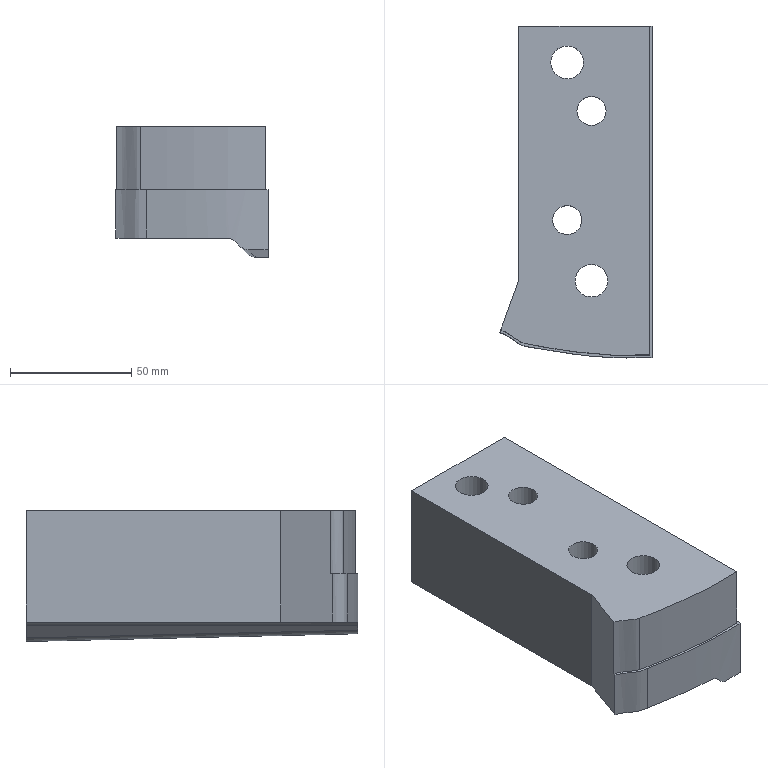Part | NX | features solid 2 | 1 solid | 30 faces | box 62.75 x 136.771 x 54 mm | volume 322596 mm3 | plane 16 | cylinder 10 | spline 4 | commonest cylinder face diameters 10 x2 12 x2 13 x2 13.5 x2 19.5 x2
STEP:
#1=CARTESIAN_POINT('',(-125.,123.027,40.));
#2=VERTEX_POINT('',#1);
#3=CARTESIAN_POINT('',(-125.,123.027,-6.));
#4=VERTEX_POINT('',#3);
#5=CARTESIAN_POINT('',(-125.,123.027,23.));
#6=DIRECTION('',(0.,0.,-1.));
#7=VECTOR('',#6,1000.);
#8=LINE('',#5,#7);
#9=EDGE_CURVE('',#2,#4,#8,.T.);
#10=ORIENTED_EDGE('',*,*,#9,.F.);
#11=CARTESIAN_POINT('',(-125.,228.,40.));
#12=VERTEX_POINT('',#11);
#13=CARTESIAN_POINT('',(-125.,35.09,40.));
#14=DIRECTION('',(0.,1.,0.));
#15=VECTOR('',#14,1000.);
#16=LINE('',#13,#15);
#17=EDGE_CURVE('',#2,#12,#16,.T.);
#18=ORIENTED_EDGE('',*,*,#17,.T.);
#19=CARTESIAN_POINT('',(-125.,228.,-6.));
#20=VERTEX_POINT('',#19);
#21=CARTESIAN_POINT('',(-125.,228.,-206.));
#22=DIRECTION('',(0.,0.,1.));
#23=VECTOR('',#22,1000.);
#24=LINE('',#21,#23);
#25=EDGE_CURVE('',#20,#12,#24,.T.);
#26=ORIENTED_EDGE('',*,*,#25,.F.);
#27=CARTESIAN_POINT('',(-125.,-222.,-6.));
#28=DIRECTION('',(0.,-1.,0.));
#29=VECTOR('',#28,1000.);
#30=LINE('',#27,#29);
#31=EDGE_CURVE('',#20,#4,#30,.T.);
#32=ORIENTED_EDGE('',*,*,#31,.T.);
#33=EDGE_LOOP('',(#10,#18,#26,#32));
#34=FACE_BOUND('',#33,.T.);
#35=CARTESIAN_POINT('',(-125.,163.62,23.));
#36=DIRECTION('',(1.,0.,0.));
#37=DIRECTION('',(0.,0.,-1.));
#38=AXIS2_PLACEMENT_3D('',#35,#36,#37);
#39=PLANE('',#38);
#40=ADVANCED_FACE('',(#34),#39,.F.);
#41=CARTESIAN_POINT('',(-71.,92.393,40.));
#42=VERTEX_POINT('',#41);
#43=CARTESIAN_POINT('',(-122.771,97.196,40.));
#44=VERTEX_POINT('',#43);
#45=CARTESIAN_POINT('',(-71.,92.393,40.));
#46=CARTESIAN_POINT('',(-75.359,92.271,40.));
#47=CARTESIAN_POINT('',(-84.076,92.056,40.));
#48=CARTESIAN_POINT('',(-97.043,93.007,40.));
#49=CARTESIAN_POINT('',(-109.924,94.861,40.));
#50=CARTESIAN_POINT('',(-118.523,96.209,40.));
#51=CARTESIAN_POINT('',(-122.771,97.196,40.));
#52=B_SPLINE_CURVE_WITH_KNOTS('',3,(#45,#46,#47,#48,#49,#50,#51),.UNSPECIFIED.,.F.,.F.,(4,1,1,1,4),(0.,0.013,0.026,0.039,0.052),.UNSPECIFIED.);
#53=EDGE_CURVE('',#42,#44,#52,.T.);
#54=ORIENTED_EDGE('',*,*,#53,.F.);
#55=CARTESIAN_POINT('',(-71.,228.,40.));
#56=VERTEX_POINT('',#55);
#57=CARTESIAN_POINT('',(-71.,35.09,40.));
#58=DIRECTION('',(0.,1.,0.));
#59=VECTOR('',#58,1000.);
#60=LINE('',#57,#59);
#61=EDGE_CURVE('',#42,#56,#60,.T.);
#62=ORIENTED_EDGE('',*,*,#61,.T.);
#63=CARTESIAN_POINT('',(-415.478,228.,40.));
#64=DIRECTION('',(1.,0.,0.));
#65=VECTOR('',#64,1000.);
#66=LINE('',#63,#65);
#67=EDGE_CURVE('',#12,#56,#66,.T.);
#68=ORIENTED_EDGE('',*,*,#67,.F.);
#69=ORIENTED_EDGE('',*,*,#17,.F.);
#70=CARTESIAN_POINT('',(-132.408,102.674,40.));
#71=VERTEX_POINT('',#70);
#72=CARTESIAN_POINT('',(-187.242,-47.981,40.));
#73=DIRECTION('',(0.342,0.9397,0.));
#74=VECTOR('',#73,1000.);
#75=LINE('',#72,#74);
#76=EDGE_CURVE('',#71,#2,#75,.T.);
#77=ORIENTED_EDGE('',*,*,#76,.F.);
#78=CARTESIAN_POINT('',(-122.771,97.196,40.));
#79=CARTESIAN_POINT('',(-124.596,97.621,40.));
#80=CARTESIAN_POINT('',(-126.742,99.529,40.));
#81=CARTESIAN_POINT('',(-129.792,101.652,40.));
#82=CARTESIAN_POINT('',(-131.523,102.356,40.));
#83=CARTESIAN_POINT('',(-132.408,102.674,40.));
#84=B_SPLINE_CURVE_WITH_KNOTS('',3,(#78,#79,#80,#81,#82,#83),.UNSPECIFIED.,.F.,.F.,(4,1,1,4),(0.,0.00551,0.008265,0.01102),.UNSPECIFIED.);
#85=EDGE_CURVE('',#44,#71,#84,.T.);
#86=ORIENTED_EDGE('',*,*,#85,.F.);
#87=EDGE_LOOP('',(#54,#62,#68,#69,#77,#86));
#88=FACE_BOUND('',#87,.T.);
#89=CARTESIAN_POINT('',(-89.,193.,40.));
#90=VERTEX_POINT('',#89);
#91=CARTESIAN_POINT('',(-95.,193.,40.));
#92=DIRECTION('',(0.,0.,1.));
#93=DIRECTION('',(1.,0.,0.));
#94=AXIS2_PLACEMENT_3D('',#91,#92,#93);
#95=CIRCLE('',#94,6.);
#96=EDGE_CURVE('',#90,#90,#95,.T.);
#97=ORIENTED_EDGE('',*,*,#96,.F.);
#98=EDGE_LOOP('',(#97));
#99=FACE_BOUND('',#98,.T.);
#100=CARTESIAN_POINT('',(-99.,148.,40.));
#101=VERTEX_POINT('',#100);
#102=CARTESIAN_POINT('',(-105.,148.,40.));
#103=DIRECTION('',(0.,0.,1.));
#104=DIRECTION('',(1.,0.,0.));
#105=AXIS2_PLACEMENT_3D('',#102,#103,#104);
#106=CIRCLE('',#105,6.);
#107=EDGE_CURVE('',#101,#101,#106,.T.);
#108=ORIENTED_EDGE('',*,*,#107,.F.);
#109=EDGE_LOOP('',(#108));
#110=FACE_BOUND('',#109,.T.);
#111=CARTESIAN_POINT('',(-98.25,213.,40.));
#112=VERTEX_POINT('',#111);
#113=CARTESIAN_POINT('',(-105.,213.,40.));
#114=DIRECTION('',(0.,0.,1.));
#115=DIRECTION('',(1.,0.,0.));
#116=AXIS2_PLACEMENT_3D('',#113,#114,#115);
#117=CIRCLE('',#116,6.75);
#118=EDGE_CURVE('',#112,#112,#117,.T.);
#119=ORIENTED_EDGE('',*,*,#118,.F.);
#120=EDGE_LOOP('',(#119));
#121=FACE_BOUND('',#120,.T.);
#122=CARTESIAN_POINT('',(-88.25,123.,40.));
#123=VERTEX_POINT('',#122);
#124=CARTESIAN_POINT('',(-95.,123.,40.));
#125=DIRECTION('',(0.,0.,1.));
#126=DIRECTION('',(1.,0.,0.));
#127=AXIS2_PLACEMENT_3D('',#124,#125,#126);
#128=CIRCLE('',#127,6.75);
#129=EDGE_CURVE('',#123,#123,#128,.T.);
#130=ORIENTED_EDGE('',*,*,#129,.F.);
#131=EDGE_LOOP('',(#130));
#132=FACE_BOUND('',#131,.T.);
#133=CARTESIAN_POINT('',(-415.478,35.09,40.));
#134=DIRECTION('',(0.,0.,1.));
#135=DIRECTION('',(1.,0.,0.));
#136=AXIS2_PLACEMENT_3D('',#133,#134,#135);
#137=PLANE('',#136);
#138=ADVANCED_FACE('',(#88,#99,#110,#121,#132),#137,.T.);
#139=CARTESIAN_POINT('',(-83.536,91.257,-7.464));
#140=VERTEX_POINT('',#139);
#141=CARTESIAN_POINT('',(-81.651,91.233,-9.349));
#142=VERTEX_POINT('',#141);
#143=CARTESIAN_POINT('',(-83.536,91.257,-7.464));
#144=CARTESIAN_POINT('',(-82.907,91.245,-8.093));
#145=CARTESIAN_POINT('',(-82.279,91.237,-8.721));
#146=CARTESIAN_POINT('',(-81.651,91.233,-9.349));
#147=B_SPLINE_CURVE_WITH_KNOTS('',3,(#143,#144,#145,#146),.UNSPECIFIED.,.F.,.F.,(4,4),(0.002071,0.004736),.UNSPECIFIED.);
#148=EDGE_CURVE('',#140,#142,#147,.T.);
#149=ORIENTED_EDGE('',*,*,#148,.T.);
#150=CARTESIAN_POINT('',(-78.112,91.242,-10.815));
#151=VERTEX_POINT('',#150);
#152=CARTESIAN_POINT('',(-81.651,91.233,-9.349));
#153=CARTESIAN_POINT('',(-80.717,91.226,-10.283));
#154=CARTESIAN_POINT('',(-79.433,91.228,-10.815));
#155=CARTESIAN_POINT('',(-78.112,91.242,-10.815));
#156=B_SPLINE_CURVE_WITH_KNOTS('',3,(#152,#153,#154,#155),.UNSPECIFIED.,.F.,.F.,(4,4),(0.,0.003908),.UNSPECIFIED.);
#157=EDGE_CURVE('',#142,#151,#156,.T.);
#158=ORIENTED_EDGE('',*,*,#157,.T.);
#159=CARTESIAN_POINT('',(-70.,91.421,-10.818));
#160=VERTEX_POINT('',#159);
#161=CARTESIAN_POINT('',(-78.112,91.242,-10.815));
#162=CARTESIAN_POINT('',(-75.407,91.271,-10.815));
#163=CARTESIAN_POINT('',(-72.704,91.343,-10.816));
#164=CARTESIAN_POINT('',(-70.,91.421,-10.818));
#165=B_SPLINE_CURVE_WITH_KNOTS('',3,(#161,#162,#163,#164),.UNSPECIFIED.,.F.,.F.,(4,4),(0.002073,0.01019),.UNSPECIFIED.);
#166=EDGE_CURVE('',#151,#160,#165,.T.);
#167=ORIENTED_EDGE('',*,*,#166,.T.);
#168=CARTESIAN_POINT('',(-70.,91.421,14.));
#169=VERTEX_POINT('',#168);
#170=CARTESIAN_POINT('',(-70.,91.421,1.5));
#171=DIRECTION('',(0.,0.,-1.));
#172=VECTOR('',#171,1000.);
#173=LINE('',#170,#172);
#174=EDGE_CURVE('',#169,#160,#173,.T.);
#175=ORIENTED_EDGE('',*,*,#174,.F.);
#176=CARTESIAN_POINT('',(-71.,91.392,14.));
#177=VERTEX_POINT('',#176);
#178=CARTESIAN_POINT('',(-71.,91.392,14.));
#179=CARTESIAN_POINT('',(-70.667,91.402,14.));
#180=CARTESIAN_POINT('',(-70.333,91.411,14.));
#181=CARTESIAN_POINT('',(-70.,91.421,14.));
#182=B_SPLINE_CURVE_WITH_KNOTS('',3,(#178,#179,#180,#181),.UNSPECIFIED.,.F.,.F.,(4,4),(0.04918,0.05017),.UNSPECIFIED.);
#183=EDGE_CURVE('',#177,#169,#182,.T.);
#184=ORIENTED_EDGE('',*,*,#183,.F.);
#185=CARTESIAN_POINT('',(-120.,95.579,14.));
#186=VERTEX_POINT('',#185);
#187=CARTESIAN_POINT('',(-190.231,-121.49,14.));
#188=CARTESIAN_POINT('',(-188.654,-121.152,14.));
#189=CARTESIAN_POINT('',(-185.47,-120.627,14.));
#190=CARTESIAN_POINT('',(-180.656,-120.141,14.));
#191=CARTESIAN_POINT('',(-175.882,-119.326,14.));
#192=CARTESIAN_POINT('',(-169.679,-117.528,14.));
#193=CARTESIAN_POINT('',(-162.185,-114.539,14.));
#194=CARTESIAN_POINT('',(-153.086,-111.254,14.));
#195=CARTESIAN_POINT('',(-144.031,-107.845,14.));
#196=CARTESIAN_POINT('',(-136.465,-105.061,14.));
#197=CARTESIAN_POINT('',(-130.418,-102.814,14.));
#198=CARTESIAN_POINT('',(-125.812,-101.329,14.));
#199=CARTESIAN_POINT('',(-121.306,-99.566,14.));
#200=CARTESIAN_POINT('',(-116.876,-97.626,14.));
#201=CARTESIAN_POINT('',(-112.335,-95.923,14.));
#202=CARTESIAN_POINT('',(-107.564,-95.05,14.));
#203=CARTESIAN_POINT('',(-102.756,-94.525,14.));
#204=CARTESIAN_POINT('',(-96.349,-93.771,14.));
#205=CARTESIAN_POINT('',(-89.902,-93.468,14.));
#206=CARTESIAN_POINT('',(-83.452,-93.448,14.));
#207=CARTESIAN_POINT('',(-77.002,-93.469,14.));
#208=CARTESIAN_POINT('',(-68.939,-93.411,14.));
#209=CARTESIAN_POINT('',(-56.04,-93.3,14.));
#210=CARTESIAN_POINT('',(-33.465,-93.184,14.));
#211=CARTESIAN_POINT('',(-7.666,-93.074,14.));
#212=CARTESIAN_POINT('',(14.907,-92.653,14.));
#213=CARTESIAN_POINT('',(27.794,-92.068,14.));
#214=CARTESIAN_POINT('',(40.668,-91.245,14.));
#215=CARTESIAN_POINT('',(51.917,-90.291,14.));
#216=CARTESIAN_POINT('',(61.528,-89.174,14.));
#217=CARTESIAN_POINT('',(67.939,-88.466,14.));
#218=CARTESIAN_POINT('',(79.125,-86.95,14.));
#219=CARTESIAN_POINT('',(95.161,-85.253,14.));
#220=CARTESIAN_POINT('',(114.404,-83.21,14.));
#221=CARTESIAN_POINT('',(133.568,-80.524,14.));
#222=CARTESIAN_POINT('',(152.734,-77.861,14.));
#223=CARTESIAN_POINT('',(171.916,-75.326,14.));
#224=CARTESIAN_POINT('',(191.055,-72.413,14.));
#225=CARTESIAN_POINT('',(207.17,-71.468,14.));
#226=CARTESIAN_POINT('',(219.951,-69.697,14.));
#227=CARTESIAN_POINT('',(232.724,-67.899,14.));
#228=CARTESIAN_POINT('',(248.708,-65.766,14.));
#229=CARTESIAN_POINT('',(267.87,-63.074,14.));
#230=CARTESIAN_POINT('',(287.038,-60.44,14.));
#231=CARTESIAN_POINT('',(301.448,-58.682,14.));
#232=CARTESIAN_POINT('',(310.976,-56.987,14.));
#233=CARTESIAN_POINT('',(314.916,-56.135,14.));
#234=CARTESIAN_POINT('',(318.052,-55.382,14.));
#235=CARTESIAN_POINT('',(320.39,-54.76,14.));
#236=CARTESIAN_POINT('',(322.686,-53.981,14.));
#237=CARTESIAN_POINT('',(325.595,-52.578,14.));
#238=CARTESIAN_POINT('',(328.769,-50.098,14.));
#239=CARTESIAN_POINT('',(332.247,-46.69,14.));
#240=CARTESIAN_POINT('',(335.795,-43.406,14.));
#241=CARTESIAN_POINT('',(343.661,-37.758,14.));
#242=CARTESIAN_POINT('',(355.164,-28.914,14.));
#243=CARTESIAN_POINT('',(370.422,-17.018,14.));
#244=CARTESIAN_POINT('',(383.264,-7.249,14.));
#245=CARTESIAN_POINT('',(392.416,-0.6713,14.));
#246=CARTESIAN_POINT('',(396.953,2.733,14.));
#247=CARTESIAN_POINT('',(398.886,5.372,14.));
#248=CARTESIAN_POINT('',(399.725,7.654,14.));
#249=CARTESIAN_POINT('',(399.76,10.078,14.));
#250=CARTESIAN_POINT('',(399.483,13.317,14.));
#251=CARTESIAN_POINT('',(399.712,17.34,14.));
#252=CARTESIAN_POINT('',(399.612,22.179,14.));
#253=CARTESIAN_POINT('',(399.633,31.854,14.));
#254=CARTESIAN_POINT('',(399.593,46.366,14.));
#255=CARTESIAN_POINT('',(399.637,62.491,14.));
#256=CARTESIAN_POINT('',(399.588,73.779,14.));
#257=CARTESIAN_POINT('',(399.652,79.422,14.));
#258=CARTESIAN_POINT('',(399.59,82.647,14.));
#259=CARTESIAN_POINT('',(399.564,85.065,14.));
#260=CARTESIAN_POINT('',(399.725,87.486,14.));
#261=CARTESIAN_POINT('',(399.756,89.902,14.));
#262=CARTESIAN_POINT('',(399.247,92.301,14.));
#263=CARTESIAN_POINT('',(397.362,95.008,14.));
#264=CARTESIAN_POINT('',(393.635,96.774,14.));
#265=CARTESIAN_POINT('',(389.279,98.826,14.));
#266=CARTESIAN_POINT('',(384.732,100.498,14.));
#267=CARTESIAN_POINT('',(378.765,102.95,14.));
#268=CARTESIAN_POINT('',(362.589,110.229,14.));
#269=CARTESIAN_POINT('',(344.928,118.135,14.));
#270=CARTESIAN_POINT('',(327.281,126.072,14.));
#271=CARTESIAN_POINT('',(319.932,129.381,14.));
#272=CARTESIAN_POINT('',(314.075,132.102,14.));
#273=CARTESIAN_POINT('',(309.387,133.376,14.));
#274=CARTESIAN_POINT('',(304.547,133.785,14.));
#275=CARTESIAN_POINT('',(299.716,133.401,14.));
#276=CARTESIAN_POINT('',(294.929,132.704,14.));
#277=CARTESIAN_POINT('',(288.543,131.8,14.));
#278=CARTESIAN_POINT('',(277.364,130.241,14.));
#279=CARTESIAN_POINT('',(242.2,125.552,14.));
#280=CARTESIAN_POINT('',(184.637,118.048,14.));
#281=CARTESIAN_POINT('',(120.701,109.541,14.));
#282=CARTESIAN_POINT('',(69.531,102.902,14.));
#283=CARTESIAN_POINT('',(40.777,98.94,14.));
#284=CARTESIAN_POINT('',(21.566,96.615,14.));
#285=CARTESIAN_POINT('',(8.743,95.212,14.));
#286=CARTESIAN_POINT('',(-7.301,93.575,14.));
#287=CARTESIAN_POINT('',(-26.625,92.505,14.));
#288=CARTESIAN_POINT('',(-45.971,92.017,14.));
#289=CARTESIAN_POINT('',(-62.09,91.675,14.));
#290=CARTESIAN_POINT('',(-74.987,91.256,14.));
#291=CARTESIAN_POINT('',(-84.664,91.165,14.));
#292=CARTESIAN_POINT('',(-94.319,91.781,14.));
#293=CARTESIAN_POINT('',(-103.929,92.966,14.));
#294=CARTESIAN_POINT('',(-113.495,94.403,14.));
#295=CARTESIAN_POINT('',(-119.856,95.492,14.));
#296=CARTESIAN_POINT('',(-122.997,96.222,14.));
#297=B_SPLINE_CURVE_WITH_KNOTS('',3,(#187,#188,#189,#190,#191,#192,#193,#194,#195,#196,#197,#198,#199,#200,#201,#202,#203,#204,#205,#206,#207,#208,#209,#210,#211,#212,#213,#214,#215,#216,#217,#218,#219,#220,#221,#222,#223,#224,#225,#226,#227,#228,#229,#230,#231,#232,#233,#234,#235,#236,#237,#238,#239,#240,#241,#242,#243,#244,#245,#246,#247,#248,#249,#250,#251,#252,#253,#254,#255,#256,#257,#258,#259,#260,#261,#262,#263,#264,#265,#266,#267,#268,#269,#270,#271,#272,#273,#274,#275,#276,#277,#278,#279,#280,#281,#282,#283,#284,#285,#286,#287,#288,#289,#290,#291,#292,#293,#294,#295,#296),.UNSPECIFIED.,.F.,.F.,(4,1,1,1,1,1,1,1,1,1,1,1,1,1,1,1,1,1,1,1,1,1,1,1,1,1,1,1,1,1,1,1,1,1,1,1,1,1,1,1,1,1,1,1,1,1,1,1,1,1,1,1,1,1,1,1,1,1,1,1,1,1,1,1,1,1,1,1,1,1,1,1,1,1,1,1,1,1,1,1,1,1,1,1,1,1,1,1,1,1,1,1,1,1,1,1,1,1,1,1,1,1,1,1,1,1,1,4),(0.4704,0.4724,0.4745,0.4766,0.4786,0.4828,0.4869,0.491,0.4952,0.4972,0.4993,0.5014,0.5035,0.5055,0.5076,0.5097,0.5117,0.5159,0.5179,0.52,0.5241,0.5283,0.5366,0.5531,0.5614,0.5655,0.5697,0.5779,0.58,0.5821,0.5862,0.5945,0.6028,0.611,0.6193,0.6276,0.6359,0.6441,0.6483,0.6524,0.6607,0.669,0.6772,0.6855,0.6876,0.6897,0.6907,0.6917,0.6928,0.6938,0.6959,0.6979,0.7,0.7021,0.7103,0.7186,0.7269,0.731,0.7331,0.7341,0.7352,0.7362,0.7372,0.7393,0.7414,0.7435,0.7517,0.76,0.7641,0.7662,0.7672,0.7683,0.7693,0.7703,0.7714,0.7724,0.7745,0.7766,0.7786,0.7807,0.7848,0.8014,0.8055,0.8097,0.8117,0.8138,0.8159,0.8179,0.82,0.8221,0.8262,0.8345,0.8676,0.9007,0.9172,0.9338,0.9379,0.9421,0.9503,0.9586,0.9669,0.9752,0.9793,0.9834,0.9876,0.9917,0.9959,1.),.UNSPECIFIED.);
#298=EDGE_CURVE('',#186,#177,#297,.F.);
#299=ORIENTED_EDGE('',*,*,#298,.F.);
#300=CARTESIAN_POINT('',(-120.,95.579,-6.));
#301=VERTEX_POINT('',#300);
#302=CARTESIAN_POINT('',(-120.,95.579,4.));
#303=DIRECTION('',(0.,0.,-1.));
#304=VECTOR('',#303,1000.);
#305=LINE('',#302,#304);
#306=EDGE_CURVE('',#301,#186,#305,.F.);
#307=ORIENTED_EDGE('',*,*,#306,.F.);
#308=CARTESIAN_POINT('',(-87.071,91.37,-6.));
#309=VERTEX_POINT('',#308);
#310=CARTESIAN_POINT('',(-87.071,91.37,-6.));
#311=CARTESIAN_POINT('',(-92.615,91.619,-6.));
#312=CARTESIAN_POINT('',(-100.865,92.521,-6.));
#313=CARTESIAN_POINT('',(-111.814,94.151,-6.));
#314=CARTESIAN_POINT('',(-117.279,95.039,-6.));
#315=CARTESIAN_POINT('',(-120.,95.579,-6.));
#316=B_SPLINE_CURVE_WITH_KNOTS('',3,(#310,#311,#312,#313,#314,#315),.UNSPECIFIED.,.F.,.F.,(4,1,1,4),(0.002065,0.01866,0.02696,0.03526),.UNSPECIFIED.);
#317=EDGE_CURVE('',#309,#301,#316,.T.);
#318=ORIENTED_EDGE('',*,*,#317,.F.);
#319=CARTESIAN_POINT('',(-87.071,91.37,-6.));
#320=CARTESIAN_POINT('',(-85.752,91.311,-6.));
#321=CARTESIAN_POINT('',(-84.469,91.275,-6.531));
#322=CARTESIAN_POINT('',(-83.536,91.257,-7.464));
#323=B_SPLINE_CURVE_WITH_KNOTS('',3,(#319,#320,#321,#322),.UNSPECIFIED.,.F.,.F.,(4,4),(0.,0.003906),.UNSPECIFIED.);
#324=EDGE_CURVE('',#309,#140,#323,.T.);
#325=ORIENTED_EDGE('',*,*,#324,.T.);
#326=EDGE_LOOP('',(#149,#158,#167,#175,#184,#299,#307,#318,#325));
#327=FACE_BOUND('',#326,.T.);
#328=CARTESIAN_POINT('',(-70.,91.421,14.));
#329=CARTESIAN_POINT('',(-70.,91.421,-10.967));
#330=CARTESIAN_POINT('',(-74.191,91.3,14.));
#331=CARTESIAN_POINT('',(-74.191,91.3,-10.967));
#332=CARTESIAN_POINT('',(-82.576,91.06,14.));
#333=CARTESIAN_POINT('',(-82.576,91.06,-10.967));
#334=CARTESIAN_POINT('',(-95.133,91.791,14.));
#335=CARTESIAN_POINT('',(-95.133,91.791,-10.967));
#336=CARTESIAN_POINT('',(-107.601,93.496,14.));
#337=CARTESIAN_POINT('',(-107.601,93.496,-10.967));
#338=CARTESIAN_POINT('',(-115.89,94.763,14.));
#339=CARTESIAN_POINT('',(-115.89,94.763,-10.967));
#340=CARTESIAN_POINT('',(-120.,95.579,14.));
#341=CARTESIAN_POINT('',(-120.,95.579,-10.967));
#342=B_SPLINE_SURFACE_WITH_KNOTS('',3,1,((#328,#329),(#330,#331),(#332,#333),(#334,#335),(#336,#337),(#338,#339),(#340,#341)),.SURF_OF_LINEAR_EXTRUSION.,.F.,.F.,.F.,(4,1,1,1,4),(2,2),(0.9772,0.9826,0.9879,0.9933,0.9987),(0.,1.),.UNSPECIFIED.);
#343=ADVANCED_FACE('',(#327),#342,.T.);
#344=CARTESIAN_POINT('',(-75.012,228.,-14.));
#345=VERTEX_POINT('',#344);
#346=CARTESIAN_POINT('',(-70.,228.,-14.));
#347=VERTEX_POINT('',#346);
#348=CARTESIAN_POINT('',(-90.,228.,-14.));
#349=DIRECTION('',(1.,0.,0.));
#350=VECTOR('',#349,1000.);
#351=LINE('',#348,#350);
#352=EDGE_CURVE('',#345,#347,#351,.T.);
#353=ORIENTED_EDGE('',*,*,#352,.F.);
#354=CARTESIAN_POINT('',(-78.465,228.,-12.535));
#355=VERTEX_POINT('',#354);
#356=CARTESIAN_POINT('',(-74.93,228.,-8.999));
#357=DIRECTION('',(0.,-1.,0.));
#358=DIRECTION('',(-0.7071,0.,0.7071));
#359=AXIS2_PLACEMENT_3D('',#356,#357,#358);
#360=ELLIPSE('',#359,5.003,5.);
#361=EDGE_CURVE('',#345,#355,#360,.F.);
#362=ORIENTED_EDGE('',*,*,#361,.T.);
#363=CARTESIAN_POINT('',(-83.536,228.,-7.464));
#364=VERTEX_POINT('',#363);
#365=CARTESIAN_POINT('',(-172.687,228.,81.687));
#366=DIRECTION('',(0.7071,0.,-0.7071));
#367=VECTOR('',#366,1000.);
#368=LINE('',#365,#367);
#369=EDGE_CURVE('',#355,#364,#368,.F.);
#370=ORIENTED_EDGE('',*,*,#369,.T.);
#371=CARTESIAN_POINT('',(-87.071,228.,-6.));
#372=VERTEX_POINT('',#371);
#373=CARTESIAN_POINT('',(-87.071,228.,-11.));
#374=DIRECTION('',(0.,-1.,0.));
#375=DIRECTION('',(1.,0.,0.));
#376=AXIS2_PLACEMENT_3D('',#373,#374,#375);
#377=CIRCLE('',#376,5.);
#378=EDGE_CURVE('',#364,#372,#377,.T.);
#379=ORIENTED_EDGE('',*,*,#378,.T.);
#380=CARTESIAN_POINT('',(-470.374,228.,-6.));
#381=DIRECTION('',(1.,0.,0.));
#382=VECTOR('',#381,1000.);
#383=LINE('',#380,#382);
#384=EDGE_CURVE('',#20,#372,#383,.T.);
#385=ORIENTED_EDGE('',*,*,#384,.F.);
#386=ORIENTED_EDGE('',*,*,#25,.T.);
#387=ORIENTED_EDGE('',*,*,#67,.T.);
#388=CARTESIAN_POINT('',(-71.,228.,14.));
#389=VERTEX_POINT('',#388);
#390=CARTESIAN_POINT('',(-71.,228.,14.));
#391=DIRECTION('',(0.,0.,-1.));
#392=VECTOR('',#391,1000.);
#393=LINE('',#390,#392);
#394=EDGE_CURVE('',#389,#56,#393,.F.);
#395=ORIENTED_EDGE('',*,*,#394,.F.);
#396=CARTESIAN_POINT('',(-70.,228.,14.));
#397=VERTEX_POINT('',#396);
#398=CARTESIAN_POINT('',(-70.,228.,14.));
#399=DIRECTION('',(1.,0.,0.));
#400=VECTOR('',#399,1000.);
#401=LINE('',#398,#400);
#402=EDGE_CURVE('',#389,#397,#401,.T.);
#403=ORIENTED_EDGE('',*,*,#402,.T.);
#404=CARTESIAN_POINT('',(-70.,228.,-206.));
#405=DIRECTION('',(0.,0.,-1.));
#406=VECTOR('',#405,1000.);
#407=LINE('',#404,#406);
#408=EDGE_CURVE('',#397,#347,#407,.T.);
#409=ORIENTED_EDGE('',*,*,#408,.T.);
#410=EDGE_LOOP('',(#353,#362,#370,#379,#385,#386,#387,#395,#403,#409));
#411=FACE_BOUND('',#410,.T.);
#412=CARTESIAN_POINT('',(-470.374,228.,-206.));
#413=DIRECTION('',(0.,-1.,0.));
#414=DIRECTION('',(1.,0.,0.));
#415=AXIS2_PLACEMENT_3D('',#412,#413,#414);
#416=PLANE('',#415);
#417=ADVANCED_FACE('',(#411),#416,.F.);
#418=CARTESIAN_POINT('',(-88.5,193.,-6.));
#419=VERTEX_POINT('',#418);
#420=CARTESIAN_POINT('',(-95.,193.,-6.));
#421=DIRECTION('',(0.,0.,1.));
#422=DIRECTION('',(1.,0.,0.));
#423=AXIS2_PLACEMENT_3D('',#420,#421,#422);
#424=CIRCLE('',#423,6.5);
#425=EDGE_CURVE('',#419,#419,#424,.T.);
#426=ORIENTED_EDGE('',*,*,#425,.T.);
#427=EDGE_LOOP('',(#426));
#428=FACE_BOUND('',#427,.T.);
#429=CARTESIAN_POINT('',(-98.5,148.,-6.));
#430=VERTEX_POINT('',#429);
#431=CARTESIAN_POINT('',(-105.,148.,-6.));
#432=DIRECTION('',(0.,0.,1.));
#433=DIRECTION('',(1.,0.,0.));
#434=AXIS2_PLACEMENT_3D('',#431,#432,#433);
#435=CIRCLE('',#434,6.5);
#436=EDGE_CURVE('',#430,#430,#435,.T.);
#437=ORIENTED_EDGE('',*,*,#436,.T.);
#438=EDGE_LOOP('',(#437));
#439=FACE_BOUND('',#438,.T.);
#440=CARTESIAN_POINT('',(-95.25,213.,-6.));
#441=VERTEX_POINT('',#440);
#442=CARTESIAN_POINT('',(-105.,213.,-6.));
#443=DIRECTION('',(0.,0.,1.));
#444=DIRECTION('',(1.,0.,0.));
#445=AXIS2_PLACEMENT_3D('',#442,#443,#444);
#446=CIRCLE('',#445,9.75);
#447=EDGE_CURVE('',#441,#441,#446,.T.);
#448=ORIENTED_EDGE('',*,*,#447,.T.);
#449=EDGE_LOOP('',(#448));
#450=FACE_BOUND('',#449,.T.);
#451=ORIENTED_EDGE('',*,*,#384,.T.);
#452=CARTESIAN_POINT('',(-87.071,128.674,-6.));
#453=VERTEX_POINT('',#452);
#454=CARTESIAN_POINT('',(-87.071,-222.,-6.));
#455=DIRECTION('',(0.,1.,0.));
#456=VECTOR('',#455,1000.);
#457=LINE('',#454,#456);
#458=EDGE_CURVE('',#372,#453,#457,.F.);
#459=ORIENTED_EDGE('',*,*,#458,.T.);
#460=CARTESIAN_POINT('',(-87.071,117.326,-6.));
#461=VERTEX_POINT('',#460);
#462=CARTESIAN_POINT('',(-95.,123.,-6.));
#463=DIRECTION('',(0.,0.,1.));
#464=DIRECTION('',(1.,0.,0.));
#465=AXIS2_PLACEMENT_3D('',#462,#463,#464);
#466=CIRCLE('',#465,9.75);
#467=EDGE_CURVE('',#453,#461,#466,.T.);
#468=ORIENTED_EDGE('',*,*,#467,.T.);
#469=CARTESIAN_POINT('',(-87.071,-222.,-6.));
#470=DIRECTION('',(0.,1.,0.));
#471=VECTOR('',#470,1000.);
#472=LINE('',#469,#471);
#473=EDGE_CURVE('',#461,#309,#472,.F.);
#474=ORIENTED_EDGE('',*,*,#473,.T.);
#475=ORIENTED_EDGE('',*,*,#317,.T.);
#476=CARTESIAN_POINT('',(-120.,95.526,-6.));
#477=VERTEX_POINT('',#476);
#478=CARTESIAN_POINT('',(-120.,163.62,-6.));
#479=DIRECTION('',(0.,1.,0.));
#480=VECTOR('',#479,1000.);
#481=LINE('',#478,#480);
#482=EDGE_CURVE('',#301,#477,#481,.F.);
#483=ORIENTED_EDGE('',*,*,#482,.T.);
#484=CARTESIAN_POINT('',(-132.75,101.734,-6.));
#485=VERTEX_POINT('',#484);
#486=CARTESIAN_POINT('',(-132.75,101.734,-6.));
#487=CARTESIAN_POINT('',(-131.611,101.325,-6.));
#488=CARTESIAN_POINT('',(-129.429,100.341,-6.));
#489=CARTESIAN_POINT('',(-126.658,98.038,-6.));
#490=CARTESIAN_POINT('',(-124.144,96.413,-6.));
#491=CARTESIAN_POINT('',(-121.752,95.948,-6.));
#492=CARTESIAN_POINT('',(-120.587,95.662,-6.));
#493=CARTESIAN_POINT('',(-120.,95.526,-6.));
#494=B_SPLINE_CURVE_WITH_KNOTS('',3,(#486,#487,#488,#489,#490,#491,#492,#493),.UNSPECIFIED.,.F.,.F.,(4,1,1,1,1,4),(0.,0.003565,0.00713,0.0107,0.01248,0.01426),.UNSPECIFIED.);
#495=EDGE_CURVE('',#485,#477,#494,.T.);
#496=ORIENTED_EDGE('',*,*,#495,.F.);
#497=CARTESIAN_POINT('',(-276.291,-292.643,-6.));
#498=DIRECTION('',(-0.342,-0.9397,0.));
#499=VECTOR('',#498,1000.);
#500=LINE('',#497,#499);
#501=EDGE_CURVE('',#485,#4,#500,.F.);
#502=ORIENTED_EDGE('',*,*,#501,.T.);
#503=ORIENTED_EDGE('',*,*,#31,.F.);
#504=EDGE_LOOP('',(#451,#459,#468,#474,#475,#483,#496,#502,#503));
#505=FACE_BOUND('',#504,.T.);
#506=CARTESIAN_POINT('',(-470.381,-222.,-6.));
#507=DIRECTION('',(0.,0.,-1.));
#508=DIRECTION('',(-1.,0.,0.));
#509=AXIS2_PLACEMENT_3D('',#506,#507,#508);
#510=PLANE('',#509);
#511=ADVANCED_FACE('',(#428,#439,#450,#505),#510,.T.);
#512=ORIENTED_EDGE('',*,*,#408,.F.);
#513=CARTESIAN_POINT('',(-70.,99.381,14.));
#514=DIRECTION('',(0.,-1.,0.));
#515=VECTOR('',#514,1000.);
#516=LINE('',#513,#515);
#517=EDGE_CURVE('',#397,#169,#516,.T.);
#518=ORIENTED_EDGE('',*,*,#517,.T.);
#519=ORIENTED_EDGE('',*,*,#174,.T.);
#520=CARTESIAN_POINT('',(-70.,99.24,-11.));
#521=DIRECTION('',(0.,0.9997,-0.02329));
#522=VECTOR('',#521,1000.);
#523=LINE('',#520,#522);
#524=EDGE_CURVE('',#160,#347,#523,.T.);
#525=ORIENTED_EDGE('',*,*,#524,.T.);
#526=EDGE_LOOP('',(#512,#518,#519,#525));
#527=FACE_BOUND('',#526,.T.);
#528=CARTESIAN_POINT('',(-70.,99.381,-66.));
#529=DIRECTION('',(-1.,0.,0.));
#530=DIRECTION('',(0.,0.,1.));
#531=AXIS2_PLACEMENT_3D('',#528,#529,#530);
#532=PLANE('',#531);
#533=ADVANCED_FACE('',(#527),#532,.F.);
#534=CARTESIAN_POINT('',(-71.,92.393,14.));
#535=VERTEX_POINT('',#534);
#536=CARTESIAN_POINT('',(-71.,99.24,14.));
#537=DIRECTION('',(0.,1.,0.));
#538=VECTOR('',#537,1000.);
#539=LINE('',#536,#538);
#540=EDGE_CURVE('',#535,#389,#539,.T.);
#541=ORIENTED_EDGE('',*,*,#540,.F.);
#542=CARTESIAN_POINT('',(-122.771,97.196,14.));
#543=VERTEX_POINT('',#542);
#544=CARTESIAN_POINT('',(-71.,92.393,14.));
#545=CARTESIAN_POINT('',(-75.361,92.271,14.));
#546=CARTESIAN_POINT('',(-84.059,92.056,14.));
#547=CARTESIAN_POINT('',(-97.021,93.004,14.));
#548=CARTESIAN_POINT('',(-109.964,94.866,14.));
#549=CARTESIAN_POINT('',(-118.57,96.22,14.));
#550=CARTESIAN_POINT('',(-122.771,97.196,14.));
#551=B_SPLINE_CURVE_WITH_KNOTS('',3,(#544,#545,#546,#547,#548,#549,#550),.UNSPECIFIED.,.F.,.F.,(4,1,1,1,4),(0.9776,0.9832,0.9888,0.9944,1.),.UNSPECIFIED.);
#552=EDGE_CURVE('',#535,#543,#551,.T.);
#553=ORIENTED_EDGE('',*,*,#552,.T.);
#554=CARTESIAN_POINT('',(-132.408,102.674,14.));
#555=VERTEX_POINT('',#554);
#556=CARTESIAN_POINT('',(-122.771,97.196,14.));
#557=CARTESIAN_POINT('',(-123.535,97.374,14.));
#558=CARTESIAN_POINT('',(-125.017,98.103,14.));
#559=CARTESIAN_POINT('',(-127.224,99.818,14.));
#560=CARTESIAN_POINT('',(-129.616,101.576,14.));
#561=CARTESIAN_POINT('',(-131.495,102.346,14.));
#562=CARTESIAN_POINT('',(-132.408,102.674,14.));
#563=B_SPLINE_CURVE_WITH_KNOTS('',3,(#556,#557,#558,#559,#560,#561,#562),.UNSPECIFIED.,.F.,.F.,(4,1,1,1,4),(0.,0.001207,0.002413,0.00362,0.004827),.UNSPECIFIED.);
#564=EDGE_CURVE('',#543,#555,#563,.T.);
#565=ORIENTED_EDGE('',*,*,#564,.T.);
#566=CARTESIAN_POINT('',(-132.75,101.734,14.));
#567=VERTEX_POINT('',#566);
#568=CARTESIAN_POINT('',(-211.217,-113.852,14.));
#569=DIRECTION('',(-0.342,-0.9397,0.));
#570=VECTOR('',#569,1000.);
#571=LINE('',#568,#570);
#572=EDGE_CURVE('',#555,#567,#571,.T.);
#573=ORIENTED_EDGE('',*,*,#572,.T.);
#574=CARTESIAN_POINT('',(-120.,95.526,14.));
#575=VERTEX_POINT('',#574);
#576=CARTESIAN_POINT('',(-112.285,93.733,14.));
#577=CARTESIAN_POINT('',(-115.856,94.563,14.));
#578=CARTESIAN_POINT('',(-119.426,95.392,14.));
#579=CARTESIAN_POINT('',(-122.997,96.222,14.));
#580=CARTESIAN_POINT('',(-124.392,96.546,14.));
#581=CARTESIAN_POINT('',(-126.827,98.157,14.));
#582=CARTESIAN_POINT('',(-130.155,100.898,14.));
#583=CARTESIAN_POINT('',(-134.281,102.244,14.));
#584=CARTESIAN_POINT('',(-139.679,104.141,14.));
#585=CARTESIAN_POINT('',(-146.371,106.694,14.));
#586=CARTESIAN_POINT('',(-154.427,109.679,14.));
#587=CARTESIAN_POINT('',(-161.126,112.208,14.));
#588=CARTESIAN_POINT('',(-165.815,113.972,14.));
#589=CARTESIAN_POINT('',(-168.494,114.99,14.));
#590=CARTESIAN_POINT('',(-171.216,115.884,14.));
#591=CARTESIAN_POINT('',(-174.721,116.613,14.));
#592=CARTESIAN_POINT('',(-178.987,117.19,14.));
#593=CARTESIAN_POINT('',(-183.249,117.724,14.));
#594=CARTESIAN_POINT('',(-191.788,118.655,14.));
#595=CARTESIAN_POINT('',(-204.643,119.63,14.));
#596=CARTESIAN_POINT('',(-218.911,120.84,14.));
#597=CARTESIAN_POINT('',(-228.851,122.152,14.));
#598=CARTESIAN_POINT('',(-234.551,122.715,14.));
#599=CARTESIAN_POINT('',(-238.829,123.073,14.));
#600=CARTESIAN_POINT('',(-243.12,123.479,14.));
#601=CARTESIAN_POINT('',(-248.75,124.526,14.));
#602=CARTESIAN_POINT('',(-255.34,127.421,14.));
#603=CARTESIAN_POINT('',(-261.873,130.381,14.));
#604=CARTESIAN_POINT('',(-265.989,133.26,14.));
#605=CARTESIAN_POINT('',(-268.199,135.082,14.));
#606=CARTESIAN_POINT('',(-270.393,136.924,14.));
#607=CARTESIAN_POINT('',(-273.148,139.209,14.));
#608=CARTESIAN_POINT('',(-277.472,142.965,14.));
#609=CARTESIAN_POINT('',(-282.708,147.853,14.));
#610=CARTESIAN_POINT('',(-289.411,153.233,14.));
#611=CARTESIAN_POINT('',(-298.398,160.336,14.));
#612=CARTESIAN_POINT('',(-314.207,172.665,14.));
#613=CARTESIAN_POINT('',(-330.339,184.575,14.));
#614=CARTESIAN_POINT('',(-343.963,195.04,14.));
#615=CARTESIAN_POINT('',(-350.855,200.194,14.));
#616=CARTESIAN_POINT('',(-355.804,205.388,14.));
#617=CARTESIAN_POINT('',(-359.395,208.889,14.));
#618=CARTESIAN_POINT('',(-361.592,210.724,14.));
#619=CARTESIAN_POINT('',(-363.291,212.042,14.));
#620=CARTESIAN_POINT('',(-364.964,213.384,14.));
#621=CARTESIAN_POINT('',(-366.621,214.773,14.));
#622=CARTESIAN_POINT('',(-368.75,215.407,14.));
#623=CARTESIAN_POINT('',(-370.894,214.756,14.));
#624=CARTESIAN_POINT('',(-372.124,213.383,14.));
#625=CARTESIAN_POINT('',(-372.711,212.074,14.));
#626=CARTESIAN_POINT('',(-373.494,210.073,14.));
#627=CARTESIAN_POINT('',(-374.087,207.63,14.));
#628=CARTESIAN_POINT('',(-375.074,204.941,14.));
#629=CARTESIAN_POINT('',(-375.964,202.22,14.));
#630=CARTESIAN_POINT('',(-377.061,198.808,14.));
#631=CARTESIAN_POINT('',(-378.358,194.734,14.));
#632=CARTESIAN_POINT('',(-379.476,191.261,14.));
#633=CARTESIAN_POINT('',(-381.61,189.247,14.));
#634=CARTESIAN_POINT('',(-384.401,188.338,14.));
#635=CARTESIAN_POINT('',(-387.982,189.153,14.));
#636=CARTESIAN_POINT('',(-392.089,190.337,14.));
#637=CARTESIAN_POINT('',(-397.637,191.766,14.));
#638=CARTESIAN_POINT('',(-402.142,192.907,14.));
#639=CARTESIAN_POINT('',(-405.767,193.016,14.));
#640=CARTESIAN_POINT('',(-406.752,192.482,14.));
#641=CARTESIAN_POINT('',(-407.204,191.679,14.));
#642=CARTESIAN_POINT('',(-407.355,190.978,14.));
#643=CARTESIAN_POINT('',(-407.778,189.239,14.));
#644=CARTESIAN_POINT('',(-409.476,182.099,14.));
#645=CARTESIAN_POINT('',(-411.921,172.376,14.));
#646=CARTESIAN_POINT('',(-414.76,162.76,14.));
#647=CARTESIAN_POINT('',(-416.63,157.346,14.));
#648=CARTESIAN_POINT('',(-418.178,153.337,14.));
#649=CARTESIAN_POINT('',(-420.236,149.537,14.));
#650=CARTESIAN_POINT('',(-423.236,146.416,14.));
#651=CARTESIAN_POINT('',(-426.787,143.984,14.));
#652=CARTESIAN_POINT('',(-431.478,140.7,14.));
#653=CARTESIAN_POINT('',(-437.23,136.434,14.));
#654=CARTESIAN_POINT('',(-444.283,131.521,14.));
#655=CARTESIAN_POINT('',(-450.102,127.369,14.));
#656=CARTESIAN_POINT('',(-454.183,123.24,14.));
#657=CARTESIAN_POINT('',(-456.026,120.178,14.));
#658=CARTESIAN_POINT('',(-456.869,117.432,14.));
#659=CARTESIAN_POINT('',(-457.557,114.647,14.));
#660=CARTESIAN_POINT('',(-458.426,111.177,14.));
#661=CARTESIAN_POINT('',(-459.295,107.705,14.));
#662=CARTESIAN_POINT('',(-460.068,104.944,14.));
#663=CARTESIAN_POINT('',(-460.556,102.852,14.));
#664=CARTESIAN_POINT('',(-460.759,100.705,14.));
#665=CARTESIAN_POINT('',(-460.539,97.842,14.));
#666=CARTESIAN_POINT('',(-458.816,93.054,14.));
#667=CARTESIAN_POINT('',(-454.37,88.976,14.));
#668=CARTESIAN_POINT('',(-449.483,87.695,14.));
#669=CARTESIAN_POINT('',(-446.657,87.236,14.));
#670=CARTESIAN_POINT('',(-443.828,86.787,14.));
#671=CARTESIAN_POINT('',(-440.31,86.125,14.));
#672=CARTESIAN_POINT('',(-434.679,85.08,14.));
#673=CARTESIAN_POINT('',(-427.604,83.939,14.));
#674=CARTESIAN_POINT('',(-420.684,82.057,14.));
#675=CARTESIAN_POINT('',(-415.851,80.778,14.));
#676=CARTESIAN_POINT('',(-413.367,80.304,14.));
#677=CARTESIAN_POINT('',(-412.158,79.475,14.));
#678=CARTESIAN_POINT('',(-411.532,78.587,14.));
#679=CARTESIAN_POINT('',(-411.333,77.527,14.));
#680=CARTESIAN_POINT('',(-411.398,76.071,14.));
#681=CARTESIAN_POINT('',(-411.844,73.616,14.));
#682=CARTESIAN_POINT('',(-412.388,68.624,14.));
#683=CARTESIAN_POINT('',(-413.428,61.542,14.));
#684=CARTESIAN_POINT('',(-414.451,50.13,14.));
#685=CARTESIAN_POINT('',(-415.942,30.138,14.));
#686=CARTESIAN_POINT('',(-416.835,1.497,14.));
#687=CARTESIAN_POINT('',(-415.947,-27.14,14.));
#688=CARTESIAN_POINT('',(-414.318,-47.126,14.));
#689=CARTESIAN_POINT('',(-413.277,-56.375,14.));
#690=CARTESIAN_POINT('',(-412.75,-60.639,14.));
#691=CARTESIAN_POINT('',(-412.511,-62.774,14.));
#692=CARTESIAN_POINT('',(-412.138,-64.888,14.));
#693=CARTESIAN_POINT('',(-411.199,-69.083,14.));
#694=CARTESIAN_POINT('',(-410.509,-72.962,14.));
#695=CARTESIAN_POINT('',(-409.724,-76.453,14.));
#696=CARTESIAN_POINT('',(-409.446,-77.862,14.));
#697=CARTESIAN_POINT('',(-409.727,-79.695,14.));
#698=CARTESIAN_POINT('',(-410.96,-81.089,14.));
#699=CARTESIAN_POINT('',(-412.257,-81.717,14.));
#700=CARTESIAN_POINT('',(-414.338,-82.265,14.));
#701=CARTESIAN_POINT('',(-417.449,-83.095,14.));
#702=CARTESIAN_POINT('',(-422.943,-84.715,14.));
#703=CARTESIAN_POINT('',(-429.89,-86.483,14.));
#704=CARTESIAN_POINT('',(-438.395,-87.724,14.));
#705=CARTESIAN_POINT('',(-445.478,-88.761,14.));
#706=CARTESIAN_POINT('',(-451.053,-90.196,14.));
#707=CARTESIAN_POINT('',(-456.021,-93.16,14.));
#708=CARTESIAN_POINT('',(-460.459,-99.179,14.));
#709=CARTESIAN_POINT('',(-460.609,-106.618,14.));
#710=CARTESIAN_POINT('',(-458.817,-112.069,14.));
#711=CARTESIAN_POINT('',(-457.691,-116.214,14.));
#712=CARTESIAN_POINT('',(-456.643,-120.377,14.));
#713=CARTESIAN_POINT('',(-454.688,-125.83,14.));
#714=CARTESIAN_POINT('',(-450.288,-129.768,14.));
#715=CARTESIAN_POINT('',(-446.15,-132.56,14.));
#716=CARTESIAN_POINT('',(-443.768,-134.151,14.));
#717=CARTESIAN_POINT('',(-441.987,-135.352,14.));
#718=CARTESIAN_POINT('',(-440.183,-136.518,14.));
#719=CARTESIAN_POINT('',(-437.722,-137.982,14.));
#720=CARTESIAN_POINT('',(-434.578,-139.696,14.));
#721=CARTESIAN_POINT('',(-431.016,-142.118,14.));
#722=CARTESIAN_POINT('',(-427.923,-145.11,14.));
#723=CARTESIAN_POINT('',(-425.28,-147.528,14.));
#724=CARTESIAN_POINT('',(-422.996,-149.255,14.));
#725=CARTESIAN_POINT('',(-420.694,-150.963,14.));
#726=CARTESIAN_POINT('',(-418.103,-153.445,14.));
#727=CARTESIAN_POINT('',(-414.699,-158.081,14.));
#728=CARTESIAN_POINT('',(-411.818,-164.69,14.));
#729=CARTESIAN_POINT('',(-409.69,-173.02,14.));
#730=CARTESIAN_POINT('',(-407.349,-181.283,14.));
#731=CARTESIAN_POINT('',(-405.436,-188.189,14.));
#732=CARTESIAN_POINT('',(-404.277,-192.687,14.));
#733=CARTESIAN_POINT('',(-403.731,-194.774,14.));
#734=CARTESIAN_POINT('',(-402.911,-195.983,14.));
#735=CARTESIAN_POINT('',(-401.476,-196.55,14.));
#736=CARTESIAN_POINT('',(-400.058,-196.272,14.));
#737=CARTESIAN_POINT('',(-398.677,-195.897,14.));
#738=CARTESIAN_POINT('',(-396.258,-195.238,14.));
#739=CARTESIAN_POINT('',(-392.822,-194.236,14.));
#740=CARTESIAN_POINT('',(-389.356,-193.338,14.));
#741=CARTESIAN_POINT('',(-386.595,-192.576,14.));
#742=CARTESIAN_POINT('',(-383.879,-191.694,14.));
#743=CARTESIAN_POINT('',(-381.029,-191.005,14.));
#744=CARTESIAN_POINT('',(-378.195,-191.605,14.));
#745=CARTESIAN_POINT('',(-375.647,-193.039,14.));
#746=CARTESIAN_POINT('',(-373.775,-196.061,14.));
#747=CARTESIAN_POINT('',(-372.459,-200.297,14.));
#748=CARTESIAN_POINT('',(-370.755,-204.215,14.));
#749=CARTESIAN_POINT('',(-369.584,-207.601,14.));
#750=CARTESIAN_POINT('',(-368.811,-210.358,14.));
#751=CARTESIAN_POINT('',(-368.284,-212.445,14.));
#752=CARTESIAN_POINT('',(-367.403,-214.035,14.));
#753=CARTESIAN_POINT('',(-366.332,-215.009,14.));
#754=CARTESIAN_POINT('',(-364.997,-215.589,14.));
#755=CARTESIAN_POINT('',(-363.147,-215.431,14.));
#756=CARTESIAN_POINT('',(-361.272,-214.331,14.));
#757=CARTESIAN_POINT('',(-359.608,-212.974,14.));
#758=CARTESIAN_POINT('',(-356.215,-210.34,14.));
#759=CARTESIAN_POINT('',(-349.028,-204.423,14.));
#760=CARTESIAN_POINT('',(-337.771,-195.573,14.));
#761=CARTESIAN_POINT('',(-324.236,-184.984,14.));
#762=CARTESIAN_POINT('',(-313.055,-176.037,14.));
#763=CARTESIAN_POINT('',(-304.322,-168.623,14.));
#764=CARTESIAN_POINT('',(-297.827,-162.998,14.));
#765=CARTESIAN_POINT('',(-291.244,-157.477,14.));
#766=CARTESIAN_POINT('',(-284.555,-152.085,14.));
#767=CARTESIAN_POINT('',(-277.805,-146.768,14.));
#768=CARTESIAN_POINT('',(-271.113,-141.381,14.));
#769=CARTESIAN_POINT('',(-264.538,-135.852,14.));
#770=CARTESIAN_POINT('',(-257.668,-130.656,14.));
#771=CARTESIAN_POINT('',(-251.187,-127.53,14.));
#772=CARTESIAN_POINT('',(-245.74,-125.755,14.));
#773=CARTESIAN_POINT('',(-241.581,-124.657,14.));
#774=CARTESIAN_POINT('',(-237.367,-123.812,14.));
#775=CARTESIAN_POINT('',(-231.672,-123.168,14.));
#776=CARTESIAN_POINT('',(-224.501,-123.191,14.));
#777=CARTESIAN_POINT('',(-215.929,-122.567,14.));
#778=CARTESIAN_POINT('',(-208.768,-122.461,14.));
#779=CARTESIAN_POINT('',(-203.041,-122.532,14.));
#780=CARTESIAN_POINT('',(-198.743,-122.639,14.));
#781=CARTESIAN_POINT('',(-194.457,-122.273,14.));
#782=CARTESIAN_POINT('',(-191.639,-121.752,14.));
#783=CARTESIAN_POINT('',(-190.231,-121.49,14.));
#784=B_SPLINE_CURVE_WITH_KNOTS('',3,(#576,#577,#578,#579,#580,#581,#582,#583,#584,#585,#586,#587,#588,#589,#590,#591,#592,#593,#594,#595,#596,#597,#598,#599,#600,#601,#602,#603,#604,#605,#606,#607,#608,#609,#610,#611,#612,#613,#614,#615,#616,#617,#618,#619,#620,#621,#622,#623,#624,#625,#626,#627,#628,#629,#630,#631,#632,#633,#634,#635,#636,#637,#638,#639,#640,#641,#642,#643,#644,#645,#646,#647,#648,#649,#650,#651,#652,#653,#654,#655,#656,#657,#658,#659,#660,#661,#662,#663,#664,#665,#666,#667,#668,#669,#670,#671,#672,#673,#674,#675,#676,#677,#678,#679,#680,#681,#682,#683,#684,#685,#686,#687,#688,#689,#690,#691,#692,#693,#694,#695,#696,#697,#698,#699,#700,#701,#702,#703,#704,#705,#706,#707,#708,#709,#710,#711,#712,#713,#714,#715,#716,#717,#718,#719,#720,#721,#722,#723,#724,#725,#726,#727,#728,#729,#730,#731,#732,#733,#734,#735,#736,#737,#738,#739,#740,#741,#742,#743,#744,#745,#746,#747,#748,#749,#750,#751,#752,#753,#754,#755,#756,#757,#758,#759,#760,#761,#762,#763,#764,#765,#766,#767,#768,#769,#770,#771,#772,#773,#774,#775,#776,#777,#778,#779,#780,#781,#782,#783),.UNSPECIFIED.,.F.,.F.,(4,3,1,1,1,1,1,1,1,1,1,1,1,1,1,1,1,1,1,1,1,1,1,1,1,1,1,1,1,1,1,1,1,1,1,1,1,1,1,1,1,1,1,1,1,1,1,1,1,1,1,1,1,1,1,1,1,1,1,1,1,1,1,1,1,1,1,1,1,1,1,1,1,1,1,1,1,1,1,1,1,1,1,1,1,1,1,1,1,1,1,1,1,1,1,1,1,1,1,1,1,1,1,1,1,1,1,1,1,1,1,1,1,1,1,1,1,1,1,1,1,1,1,1,1,1,1,1,1,1,1,1,1,1,1,1,1,1,1,1,1,1,1,1,1,1,1,1,1,1,1,1,1,1,1,1,1,1,1,1,1,1,1,1,1,1,1,1,1,1,1,1,1,1,1,1,1,1,1,1,1,1,1,1,1,1,1,1,1,1,1,1,1,1,1,1,1,1,1,1,1,1,1,4),(-0.004704,0.,0.001837,0.003675,0.005512,0.007349,0.01102,0.0147,0.01837,0.02021,0.02113,0.02205,0.02388,0.02572,0.02756,0.0294,0.03675,0.0441,0.04777,0.04961,0.05144,0.05328,0.05512,0.05879,0.06247,0.06431,0.06522,0.06614,0.06798,0.06982,0.07349,0.07717,0.08084,0.08819,0.1029,0.1066,0.1102,0.1139,0.1158,0.1167,0.1176,0.1185,0.1194,0.1203,0.1213,0.1222,0.1226,0.1231,0.1249,0.1259,0.1268,0.1286,0.1304,0.1323,0.1332,0.1341,0.136,0.1378,0.1396,0.1433,0.1438,0.1442,0.1447,0.1449,0.1451,0.147,0.1543,0.158,0.1598,0.1617,0.1635,0.1654,0.1672,0.169,0.1727,0.1764,0.1801,0.1819,0.1837,0.1846,0.1856,0.1874,0.1892,0.1902,0.1911,0.192,0.1929,0.1948,0.1984,0.2003,0.2012,0.2021,0.2039,0.2058,0.2095,0.2131,0.215,0.2159,0.2163,0.2168,0.2173,0.2177,0.2186,0.2205,0.2242,0.2278,0.2352,0.2499,0.2646,0.2719,0.2756,0.2765,0.2774,0.2784,0.2793,0.2829,0.2834,0.2839,0.2848,0.2857,0.2862,0.2866,0.2885,0.2903,0.294,0.2976,0.3013,0.3032,0.305,0.3087,0.3123,0.3142,0.316,0.3179,0.3197,0.3234,0.3252,0.3261,0.327,0.328,0.3289,0.3307,0.3326,0.3344,0.3362,0.3371,0.3381,0.3399,0.3417,0.3454,0.3491,0.3528,0.3564,0.3583,0.3587,0.3592,0.3601,0.3606,0.361,0.3619,0.3638,0.3656,0.3665,0.3675,0.3693,0.3702,0.3711,0.373,0.3748,0.3766,0.3785,0.3794,0.3803,0.3812,0.3817,0.3822,0.3831,0.384,0.3849,0.3858,0.3895,0.3969,0.4042,0.4116,0.4152,0.4189,0.4226,0.4263,0.4299,0.4336,0.4373,0.441,0.4446,0.4465,0.4483,0.4501,0.452,0.4557,0.4593,0.463,0.4648,0.4667,0.4685,0.4704),.UNSPECIFIED.);
#785=EDGE_CURVE('',#567,#575,#784,.F.);
#786=ORIENTED_EDGE('',*,*,#785,.T.);
#787=CARTESIAN_POINT('',(-120.,163.62,14.));
#788=DIRECTION('',(0.,1.,0.));
#789=VECTOR('',#788,1000.);
#790=LINE('',#787,#789);
#791=EDGE_CURVE('',#575,#186,#790,.T.);
#792=ORIENTED_EDGE('',*,*,#791,.T.);
#793=ORIENTED_EDGE('',*,*,#298,.T.);
#794=ORIENTED_EDGE('',*,*,#183,.T.);
#795=ORIENTED_EDGE('',*,*,#517,.F.);
#796=ORIENTED_EDGE('',*,*,#402,.F.);
#797=EDGE_LOOP('',(#541,#553,#565,#573,#786,#792,#793,#794,#795,#796));
#798=FACE_BOUND('',#797,.T.);
#799=CARTESIAN_POINT('',(-454.349,119.974,14.));
#800=DIRECTION('',(0.,0.,-1.));
#801=DIRECTION('',(-1.,0.,0.));
#802=AXIS2_PLACEMENT_3D('',#799,#800,#801);
#803=PLANE('',#802);
#804=ADVANCED_FACE('',(#798),#803,.F.);
#805=CARTESIAN_POINT('',(-71.,92.393,57.));
#806=DIRECTION('',(0.,0.,1.));
#807=VECTOR('',#806,1000.);
#808=LINE('',#805,#807);
#809=EDGE_CURVE('',#535,#42,#808,.T.);
#810=ORIENTED_EDGE('',*,*,#809,.F.);
#811=ORIENTED_EDGE('',*,*,#540,.T.);
#812=ORIENTED_EDGE('',*,*,#394,.T.);
#813=ORIENTED_EDGE('',*,*,#61,.F.);
#814=EDGE_LOOP('',(#810,#811,#812,#813));
#815=FACE_BOUND('',#814,.T.);
#816=CARTESIAN_POINT('',(-71.,99.24,14.));
#817=DIRECTION('',(1.,0.,0.));
#818=DIRECTION('',(0.,0.,-1.));
#819=AXIS2_PLACEMENT_3D('',#816,#817,#818);
#820=PLANE('',#819);
#821=ADVANCED_FACE('',(#815),#820,.T.);
#822=ORIENTED_EDGE('',*,*,#369,.F.);
#823=CARTESIAN_POINT('',(-81.463,99.308,-9.537));
#824=DIRECTION('',(0.02328,0.9995,-0.02328));
#825=VECTOR('',#824,1000.);
#826=LINE('',#823,#825);
#827=EDGE_CURVE('',#355,#142,#826,.F.);
#828=ORIENTED_EDGE('',*,*,#827,.T.);
#829=ORIENTED_EDGE('',*,*,#148,.F.);
#830=CARTESIAN_POINT('',(-83.536,99.24,-7.464));
#831=DIRECTION('',(0.,-1.,0.));
#832=VECTOR('',#831,1000.);
#833=LINE('',#830,#832);
#834=EDGE_CURVE('',#140,#364,#833,.F.);
#835=ORIENTED_EDGE('',*,*,#834,.T.);
#836=EDGE_LOOP('',(#822,#828,#829,#835));
#837=FACE_BOUND('',#836,.T.);
#838=CARTESIAN_POINT('',(-80.,99.24,-11.));
#839=DIRECTION('',(-0.7071,0.,-0.7071));
#840=DIRECTION('',(-0.7071,0.,0.7071));
#841=AXIS2_PLACEMENT_3D('',#838,#839,#840);
#842=PLANE('',#841);
#843=ADVANCED_FACE('',(#837),#842,.T.);
#844=ORIENTED_EDGE('',*,*,#129,.T.);
#845=EDGE_LOOP('',(#844));
#846=FACE_BOUND('',#845,.T.);
#847=CARTESIAN_POINT('',(-88.25,123.,9.));
#848=VERTEX_POINT('',#847);
#849=CARTESIAN_POINT('',(-95.,123.,9.));
#850=DIRECTION('',(0.,0.,1.));
#851=DIRECTION('',(1.,0.,0.));
#852=AXIS2_PLACEMENT_3D('',#849,#850,#851);
#853=CIRCLE('',#852,6.75);
#854=EDGE_CURVE('',#848,#848,#853,.T.);
#855=ORIENTED_EDGE('',*,*,#854,.F.);
#856=EDGE_LOOP('',(#855));
#857=FACE_BOUND('',#856,.T.);
#858=CARTESIAN_POINT('',(-95.,123.,94.));
#859=DIRECTION('',(0.,0.,1.));
#860=DIRECTION('',(1.,0.,0.));
#861=AXIS2_PLACEMENT_3D('',#858,#859,#860);
#862=CYLINDRICAL_SURFACE('',#861,6.75);
#863=ADVANCED_FACE('',(#846,#857),#862,.F.);
#864=ORIENTED_EDGE('',*,*,#854,.T.);
#865=EDGE_LOOP('',(#864));
#866=FACE_BOUND('',#865,.T.);
#867=CARTESIAN_POINT('',(-85.25,123.,9.));
#868=VERTEX_POINT('',#867);
#869=CARTESIAN_POINT('',(-95.,123.,9.));
#870=DIRECTION('',(0.,0.,1.));
#871=DIRECTION('',(1.,0.,0.));
#872=AXIS2_PLACEMENT_3D('',#869,#870,#871);
#873=CIRCLE('',#872,9.75);
#874=EDGE_CURVE('',#868,#868,#873,.T.);
#875=ORIENTED_EDGE('',*,*,#874,.F.);
#876=EDGE_LOOP('',(#875));
#877=FACE_BOUND('',#876,.T.);
#878=CARTESIAN_POINT('',(-95.,118.,9.));
#879=DIRECTION('',(0.,0.,1.));
#880=DIRECTION('',(1.,0.,0.));
#881=AXIS2_PLACEMENT_3D('',#878,#879,#880);
#882=PLANE('',#881);
#883=ADVANCED_FACE('',(#866,#877),#882,.F.);
#884=ORIENTED_EDGE('',*,*,#874,.T.);
#885=EDGE_LOOP('',(#884));
#886=FACE_BOUND('',#885,.T.);
#887=ORIENTED_EDGE('',*,*,#467,.F.);
#888=CARTESIAN_POINT('',(-87.071,128.674,-6.));
#889=CARTESIAN_POINT('',(-85.887,127.019,-6.));
#890=CARTESIAN_POINT('',(-84.613,122.988,-6.687));
#891=CARTESIAN_POINT('',(-85.888,118.98,-6.));
#892=CARTESIAN_POINT('',(-87.071,117.326,-6.));
#893=B_SPLINE_CURVE_WITH_KNOTS('',3,(#888,#889,#890,#891,#892),.UNSPECIFIED.,.F.,.F.,(4,1,4),(0.002361,0.008399,0.01444),.UNSPECIFIED.);
#894=EDGE_CURVE('',#461,#453,#893,.F.);
#895=ORIENTED_EDGE('',*,*,#894,.F.);
#896=EDGE_LOOP('',(#887,#895));
#897=FACE_BOUND('',#896,.T.);
#898=CARTESIAN_POINT('',(-95.,123.,-6.));
#899=DIRECTION('',(0.,0.,1.));
#900=DIRECTION('',(1.,0.,0.));
#901=AXIS2_PLACEMENT_3D('',#898,#899,#900);
#902=CYLINDRICAL_SURFACE('',#901,9.75);
#903=ADVANCED_FACE('',(#886,#897),#902,.F.);
#904=ORIENTED_EDGE('',*,*,#118,.T.);
#905=EDGE_LOOP('',(#904));
#906=FACE_BOUND('',#905,.T.);
#907=CARTESIAN_POINT('',(-98.25,213.,9.));
#908=VERTEX_POINT('',#907);
#909=CARTESIAN_POINT('',(-105.,213.,9.));
#910=DIRECTION('',(0.,0.,1.));
#911=DIRECTION('',(1.,0.,0.));
#912=AXIS2_PLACEMENT_3D('',#909,#910,#911);
#913=CIRCLE('',#912,6.75);
#914=EDGE_CURVE('',#908,#908,#913,.T.);
#915=ORIENTED_EDGE('',*,*,#914,.F.);
#916=EDGE_LOOP('',(#915));
#917=FACE_BOUND('',#916,.T.);
#918=CARTESIAN_POINT('',(-105.,213.,94.));
#919=DIRECTION('',(0.,0.,1.));
#920=DIRECTION('',(1.,0.,0.));
#921=AXIS2_PLACEMENT_3D('',#918,#919,#920);
#922=CYLINDRICAL_SURFACE('',#921,6.75);
#923=ADVANCED_FACE('',(#906,#917),#922,.F.);
#924=ORIENTED_EDGE('',*,*,#914,.T.);
#925=EDGE_LOOP('',(#924));
#926=FACE_BOUND('',#925,.T.);
#927=CARTESIAN_POINT('',(-95.25,213.,9.));
#928=VERTEX_POINT('',#927);
#929=CARTESIAN_POINT('',(-105.,213.,9.));
#930=DIRECTION('',(0.,0.,1.));
#931=DIRECTION('',(1.,0.,0.));
#932=AXIS2_PLACEMENT_3D('',#929,#930,#931);
#933=CIRCLE('',#932,9.75);
#934=EDGE_CURVE('',#928,#928,#933,.T.);
#935=ORIENTED_EDGE('',*,*,#934,.F.);
#936=EDGE_LOOP('',(#935));
#937=FACE_BOUND('',#936,.T.);
#938=CARTESIAN_POINT('',(-105.,213.,9.));
#939=DIRECTION('',(0.,0.,1.));
#940=DIRECTION('',(1.,0.,0.));
#941=AXIS2_PLACEMENT_3D('',#938,#939,#940);
#942=PLANE('',#941);
#943=ADVANCED_FACE('',(#926,#937),#942,.F.);
#944=ORIENTED_EDGE('',*,*,#934,.T.);
#945=EDGE_LOOP('',(#944));
#946=FACE_BOUND('',#945,.T.);
#947=ORIENTED_EDGE('',*,*,#447,.F.);
#948=EDGE_LOOP('',(#947));
#949=FACE_BOUND('',#948,.T.);
#950=CARTESIAN_POINT('',(-105.,213.,-6.));
#951=DIRECTION('',(0.,0.,1.));
#952=DIRECTION('',(1.,0.,0.));
#953=AXIS2_PLACEMENT_3D('',#950,#951,#952);
#954=CYLINDRICAL_SURFACE('',#953,9.75);
#955=ADVANCED_FACE('',(#946,#949),#954,.F.);
#956=ORIENTED_EDGE('',*,*,#107,.T.);
#957=EDGE_LOOP('',(#956));
#958=FACE_BOUND('',#957,.T.);
#959=CARTESIAN_POINT('',(-99.,148.,14.));
#960=VERTEX_POINT('',#959);
#961=CARTESIAN_POINT('',(-105.,148.,14.));
#962=DIRECTION('',(0.,0.,1.));
#963=DIRECTION('',(1.,0.,0.));
#964=AXIS2_PLACEMENT_3D('',#961,#962,#963);
#965=CIRCLE('',#964,6.);
#966=EDGE_CURVE('',#960,#960,#965,.T.);
#967=ORIENTED_EDGE('',*,*,#966,.F.);
#968=EDGE_LOOP('',(#967));
#969=FACE_BOUND('',#968,.T.);
#970=CARTESIAN_POINT('',(-105.,148.,94.));
#971=DIRECTION('',(0.,0.,1.));
#972=DIRECTION('',(1.,0.,0.));
#973=AXIS2_PLACEMENT_3D('',#970,#971,#972);
#974=CYLINDRICAL_SURFACE('',#973,6.);
#975=ADVANCED_FACE('',(#958,#969),#974,.F.);
#976=ORIENTED_EDGE('',*,*,#966,.T.);
#977=EDGE_LOOP('',(#976));
#978=FACE_BOUND('',#977,.T.);
#979=CARTESIAN_POINT('',(-98.5,148.,14.));
#980=VERTEX_POINT('',#979);
#981=CARTESIAN_POINT('',(-105.,148.,14.));
#982=DIRECTION('',(0.,0.,1.));
#983=DIRECTION('',(1.,0.,0.));
#984=AXIS2_PLACEMENT_3D('',#981,#982,#983);
#985=CIRCLE('',#984,6.5);
#986=EDGE_CURVE('',#980,#980,#985,.T.);
#987=ORIENTED_EDGE('',*,*,#986,.F.);
#988=EDGE_LOOP('',(#987));
#989=FACE_BOUND('',#988,.T.);
#990=CARTESIAN_POINT('',(-105.,148.,14.));
#991=DIRECTION('',(0.,0.,1.));
#992=DIRECTION('',(1.,0.,0.));
#993=AXIS2_PLACEMENT_3D('',#990,#991,#992);
#994=PLANE('',#993);
#995=ADVANCED_FACE('',(#978,#989),#994,.F.);
#996=ORIENTED_EDGE('',*,*,#986,.T.);
#997=EDGE_LOOP('',(#996));
#998=FACE_BOUND('',#997,.T.);
#999=ORIENTED_EDGE('',*,*,#436,.F.);
#1000=EDGE_LOOP('',(#999));
#1001=FACE_BOUND('',#1000,.T.);
#1002=CARTESIAN_POINT('',(-105.,148.,-6.));
#1003=DIRECTION('',(0.,0.,1.));
#1004=DIRECTION('',(1.,0.,0.));
#1005=AXIS2_PLACEMENT_3D('',#1002,#1003,#1004);
#1006=CYLINDRICAL_SURFACE('',#1005,6.5);
#1007=ADVANCED_FACE('',(#998,#1001),#1006,.F.);
#1008=ORIENTED_EDGE('',*,*,#96,.T.);
#1009=EDGE_LOOP('',(#1008));
#1010=FACE_BOUND('',#1009,.T.);
#1011=CARTESIAN_POINT('',(-89.,193.,14.));
#1012=VERTEX_POINT('',#1011);
#1013=CARTESIAN_POINT('',(-95.,193.,14.));
#1014=DIRECTION('',(0.,0.,1.));
#1015=DIRECTION('',(1.,0.,0.));
#1016=AXIS2_PLACEMENT_3D('',#1013,#1014,#1015);
#1017=CIRCLE('',#1016,6.);
#1018=EDGE_CURVE('',#1012,#1012,#1017,.T.);
#1019=ORIENTED_EDGE('',*,*,#1018,.F.);
#1020=EDGE_LOOP('',(#1019));
#1021=FACE_BOUND('',#1020,.T.);
#1022=CARTESIAN_POINT('',(-95.,193.,94.));
#1023=DIRECTION('',(0.,0.,1.));
#1024=DIRECTION('',(1.,0.,0.));
#1025=AXIS2_PLACEMENT_3D('',#1022,#1023,#1024);
#1026=CYLINDRICAL_SURFACE('',#1025,6.);
#1027=ADVANCED_FACE('',(#1010,#1021),#1026,.F.);
#1028=ORIENTED_EDGE('',*,*,#1018,.T.);
#1029=EDGE_LOOP('',(#1028));
#1030=FACE_BOUND('',#1029,.T.);
#1031=CARTESIAN_POINT('',(-88.5,193.,14.));
#1032=VERTEX_POINT('',#1031);
#1033=CARTESIAN_POINT('',(-95.,193.,14.));
#1034=DIRECTION('',(0.,0.,1.));
#1035=DIRECTION('',(1.,0.,0.));
#1036=AXIS2_PLACEMENT_3D('',#1033,#1034,#1035);
#1037=CIRCLE('',#1036,6.5);
#1038=EDGE_CURVE('',#1032,#1032,#1037,.T.);
#1039=ORIENTED_EDGE('',*,*,#1038,.F.);
#1040=EDGE_LOOP('',(#1039));
#1041=FACE_BOUND('',#1040,.T.);
#1042=CARTESIAN_POINT('',(-95.,193.,14.));
#1043=DIRECTION('',(0.,0.,1.));
#1044=DIRECTION('',(1.,0.,0.));
#1045=AXIS2_PLACEMENT_3D('',#1042,#1043,#1044);
#1046=PLANE('',#1045);
#1047=ADVANCED_FACE('',(#1030,#1041),#1046,.F.);
#1048=ORIENTED_EDGE('',*,*,#1038,.T.);
#1049=EDGE_LOOP('',(#1048));
#1050=FACE_BOUND('',#1049,.T.);
#1051=ORIENTED_EDGE('',*,*,#425,.F.);
#1052=EDGE_LOOP('',(#1051));
#1053=FACE_BOUND('',#1052,.T.);
#1054=CARTESIAN_POINT('',(-95.,193.,-6.));
#1055=DIRECTION('',(0.,0.,1.));
#1056=DIRECTION('',(1.,0.,0.));
#1057=AXIS2_PLACEMENT_3D('',#1054,#1055,#1056);
#1058=CYLINDRICAL_SURFACE('',#1057,6.5);
#1059=ADVANCED_FACE('',(#1050,#1053),#1058,.F.);
#1060=CARTESIAN_POINT('',(-74.927,227.969,-14.));
#1061=VERTEX_POINT('',#1060);
#1062=CARTESIAN_POINT('',(-90.812,227.869,-14.));
#1063=DIRECTION('',(1.,0.006316,0.));
#1064=VECTOR('',#1063,1000.);
#1065=LINE('',#1062,#1064);
#1066=EDGE_CURVE('',#1061,#347,#1065,.T.);
#1067=ORIENTED_EDGE('',*,*,#1066,.F.);
#1068=CARTESIAN_POINT('',(-69.929,442.658,-14.));
#1069=DIRECTION('',(0.,0.,-1.));
#1070=DIRECTION('',(-0.02329,-0.9997,0.));
#1071=AXIS2_PLACEMENT_3D('',#1068,#1069,#1070);
#1072=ELLIPSE('',#1071,214.748,5.);
#1073=EDGE_CURVE('',#1061,#345,#1072,.T.);
#1074=ORIENTED_EDGE('',*,*,#1073,.T.);
#1075=ORIENTED_EDGE('',*,*,#352,.T.);
#1076=EDGE_LOOP('',(#1067,#1074,#1075));
#1077=FACE_BOUND('',#1076,.T.);
#1078=CARTESIAN_POINT('',(-90.,99.24,-14.));
#1079=DIRECTION('',(0.,0.,-1.));
#1080=DIRECTION('',(-1.,0.,0.));
#1081=AXIS2_PLACEMENT_3D('',#1078,#1079,#1080);
#1082=PLANE('',#1081);
#1083=ADVANCED_FACE('',(#1077),#1082,.T.);
#1084=ORIENTED_EDGE('',*,*,#166,.F.);
#1085=CARTESIAN_POINT('',(-77.928,99.129,-10.999));
#1086=DIRECTION('',(-0.02328,-0.9995,0.02328));
#1087=VECTOR('',#1086,1000.);
#1088=LINE('',#1085,#1087);
#1089=EDGE_CURVE('',#151,#1061,#1088,.F.);
#1090=ORIENTED_EDGE('',*,*,#1089,.T.);
#1091=ORIENTED_EDGE('',*,*,#1066,.T.);
#1092=ORIENTED_EDGE('',*,*,#524,.F.);
#1093=EDGE_LOOP('',(#1084,#1090,#1091,#1092));
#1094=FACE_BOUND('',#1093,.T.);
#1095=CARTESIAN_POINT('',(-80.,99.177,-11.));
#1096=DIRECTION('',(-0.0001471,0.02329,0.9997));
#1097=DIRECTION('',(0.,-0.9997,0.02329));
#1098=AXIS2_PLACEMENT_3D('',#1095,#1096,#1097);
#1099=PLANE('',#1098);
#1100=ADVANCED_FACE('',(#1094),#1099,.F.);
#1101=ORIENTED_EDGE('',*,*,#552,.F.);
#1102=ORIENTED_EDGE('',*,*,#809,.T.);
#1103=ORIENTED_EDGE('',*,*,#53,.T.);
#1104=CARTESIAN_POINT('',(-122.771,97.196,14.));
#1105=DIRECTION('',(0.,0.,1.));
#1106=VECTOR('',#1105,1000.);
#1107=LINE('',#1104,#1106);
#1108=EDGE_CURVE('',#543,#44,#1107,.T.);
#1109=ORIENTED_EDGE('',*,*,#1108,.F.);
#1110=EDGE_LOOP('',(#1101,#1102,#1103,#1109));
#1111=FACE_BOUND('',#1110,.T.);
#1112=CARTESIAN_POINT('',(-71.,92.393,14.));
#1113=CARTESIAN_POINT('',(-71.,92.393,40.));
#1114=CARTESIAN_POINT('',(-75.361,92.271,14.));
#1115=CARTESIAN_POINT('',(-75.361,92.271,40.));
#1116=CARTESIAN_POINT('',(-84.059,92.056,14.));
#1117=CARTESIAN_POINT('',(-84.059,92.056,40.));
#1118=CARTESIAN_POINT('',(-97.021,93.004,14.));
#1119=CARTESIAN_POINT('',(-97.021,93.004,40.));
#1120=CARTESIAN_POINT('',(-109.964,94.866,14.));
#1121=CARTESIAN_POINT('',(-109.964,94.866,40.));
#1122=CARTESIAN_POINT('',(-118.57,96.22,14.));
#1123=CARTESIAN_POINT('',(-118.57,96.22,40.));
#1124=CARTESIAN_POINT('',(-122.771,97.196,14.));
#1125=CARTESIAN_POINT('',(-122.771,97.196,40.));
#1126=B_SPLINE_SURFACE_WITH_KNOTS('',3,1,((#1112,#1113),(#1114,#1115),(#1116,#1117),(#1118,#1119),(#1120,#1121),(#1122,#1123),(#1124,#1125)),.SURF_OF_LINEAR_EXTRUSION.,.F.,.F.,.F.,(4,1,1,1,4),(2,2),(0.9776,0.9832,0.9888,0.9944,1.),(0.,1.),.UNSPECIFIED.);
#1127=ADVANCED_FACE('',(#1111),#1126,.F.);
#1128=ORIENTED_EDGE('',*,*,#85,.T.);
#1129=CARTESIAN_POINT('',(-132.408,102.674,27.));
#1130=DIRECTION('',(0.,0.,1.));
#1131=VECTOR('',#1130,1000.);
#1132=LINE('',#1129,#1131);
#1133=EDGE_CURVE('',#71,#555,#1132,.F.);
#1134=ORIENTED_EDGE('',*,*,#1133,.T.);
#1135=ORIENTED_EDGE('',*,*,#564,.F.);
#1136=ORIENTED_EDGE('',*,*,#1108,.T.);
#1137=EDGE_LOOP('',(#1128,#1134,#1135,#1136));
#1138=FACE_BOUND('',#1137,.T.);
#1139=CARTESIAN_POINT('',(-122.771,97.196,14.));
#1140=CARTESIAN_POINT('',(-122.771,97.196,40.));
#1141=CARTESIAN_POINT('',(-123.535,97.374,14.));
#1142=CARTESIAN_POINT('',(-123.535,97.374,40.));
#1143=CARTESIAN_POINT('',(-125.017,98.103,14.));
#1144=CARTESIAN_POINT('',(-125.017,98.103,40.));
#1145=CARTESIAN_POINT('',(-127.224,99.818,14.));
#1146=CARTESIAN_POINT('',(-127.224,99.818,40.));
#1147=CARTESIAN_POINT('',(-129.616,101.576,14.));
#1148=CARTESIAN_POINT('',(-129.616,101.576,40.));
#1149=CARTESIAN_POINT('',(-131.495,102.346,14.));
#1150=CARTESIAN_POINT('',(-131.495,102.346,40.));
#1151=CARTESIAN_POINT('',(-132.408,102.674,14.));
#1152=CARTESIAN_POINT('',(-132.408,102.674,40.));
#1153=B_SPLINE_SURFACE_WITH_KNOTS('',3,1,((#1139,#1140),(#1141,#1142),(#1143,#1144),(#1145,#1146),(#1147,#1148),(#1149,#1150),(#1151,#1152)),.SURF_OF_LINEAR_EXTRUSION.,.F.,.F.,.F.,(4,1,1,1,4),(2,2),(0.,0.001207,0.002413,0.00362,0.004827),(0.,1.),.UNSPECIFIED.);
#1154=ADVANCED_FACE('',(#1138),#1153,.F.);
#1155=CARTESIAN_POINT('',(-132.75,101.734,2.42));
#1156=DIRECTION('',(0.,0.,-1.));
#1157=VECTOR('',#1156,1000.);
#1158=LINE('',#1155,#1157);
#1159=EDGE_CURVE('',#485,#567,#1158,.F.);
#1160=ORIENTED_EDGE('',*,*,#1159,.F.);
#1161=ORIENTED_EDGE('',*,*,#495,.T.);
#1162=CARTESIAN_POINT('',(-120.,95.526,2.5));
#1163=DIRECTION('',(0.,0.,-1.));
#1164=VECTOR('',#1163,1000.);
#1165=LINE('',#1162,#1164);
#1166=EDGE_CURVE('',#477,#575,#1165,.F.);
#1167=ORIENTED_EDGE('',*,*,#1166,.T.);
#1168=ORIENTED_EDGE('',*,*,#785,.F.);
#1169=EDGE_LOOP('',(#1160,#1161,#1167,#1168));
#1170=FACE_BOUND('',#1169,.T.);
#1171=CARTESIAN_POINT('',(-120.,95.526,14.));
#1172=CARTESIAN_POINT('',(-120.,95.526,-6.));
#1173=CARTESIAN_POINT('',(-120.583,95.661,14.));
#1174=CARTESIAN_POINT('',(-120.583,95.661,-6.));
#1175=CARTESIAN_POINT('',(-121.744,95.947,14.));
#1176=CARTESIAN_POINT('',(-121.744,95.947,-6.));
#1177=CARTESIAN_POINT('',(-124.109,96.401,14.));
#1178=CARTESIAN_POINT('',(-124.109,96.401,-6.));
#1179=CARTESIAN_POINT('',(-126.666,98.039,14.));
#1180=CARTESIAN_POINT('',(-126.666,98.039,-6.));
#1181=CARTESIAN_POINT('',(-129.449,100.356,14.));
#1182=CARTESIAN_POINT('',(-129.449,100.356,-6.));
#1183=CARTESIAN_POINT('',(-131.619,101.328,14.));
#1184=CARTESIAN_POINT('',(-131.619,101.328,-6.));
#1185=CARTESIAN_POINT('',(-132.75,101.734,14.));
#1186=CARTESIAN_POINT('',(-132.75,101.734,-6.));
#1187=B_SPLINE_SURFACE_WITH_KNOTS('',3,1,((#1171,#1172),(#1173,#1174),(#1175,#1176),(#1177,#1178),(#1179,#1180),(#1181,#1182),(#1183,#1184),(#1185,#1186)),.SURF_OF_LINEAR_EXTRUSION.,.F.,.F.,.F.,(4,1,1,1,1,4),(2,2),(-0.001316,-0.0005478,0.0002202,0.001756,0.003292,0.004829),(0.,1.),.UNSPECIFIED.);
#1188=ADVANCED_FACE('',(#1170),#1187,.T.);
#1189=ORIENTED_EDGE('',*,*,#482,.F.);
#1190=ORIENTED_EDGE('',*,*,#306,.T.);
#1191=ORIENTED_EDGE('',*,*,#791,.F.);
#1192=ORIENTED_EDGE('',*,*,#1166,.F.);
#1193=EDGE_LOOP('',(#1189,#1190,#1191,#1192));
#1194=FACE_BOUND('',#1193,.T.);
#1195=CARTESIAN_POINT('',(-120.,163.62,23.));
#1196=DIRECTION('',(1.,0.,0.));
#1197=DIRECTION('',(0.,0.,-1.));
#1198=AXIS2_PLACEMENT_3D('',#1195,#1196,#1197);
#1199=PLANE('',#1198);
#1200=ADVANCED_FACE('',(#1194),#1199,.T.);
#1201=ORIENTED_EDGE('',*,*,#9,.T.);
#1202=ORIENTED_EDGE('',*,*,#501,.F.);
#1203=ORIENTED_EDGE('',*,*,#1159,.T.);
#1204=ORIENTED_EDGE('',*,*,#572,.F.);
#1205=ORIENTED_EDGE('',*,*,#1133,.F.);
#1206=ORIENTED_EDGE('',*,*,#76,.T.);
#1207=EDGE_LOOP('',(#1201,#1202,#1203,#1204,#1205,#1206));
#1208=FACE_BOUND('',#1207,.T.);
#1209=CARTESIAN_POINT('',(-160.506,25.475,0.));
#1210=DIRECTION('',(0.9397,-0.342,0.));
#1211=DIRECTION('',(0.342,0.9397,0.));
#1212=AXIS2_PLACEMENT_3D('',#1209,#1210,#1211);
#1213=PLANE('',#1212);
#1214=ADVANCED_FACE('',(#1208),#1213,.F.);
#1215=ORIENTED_EDGE('',*,*,#324,.F.);
#1216=ORIENTED_EDGE('',*,*,#473,.F.);
#1217=ORIENTED_EDGE('',*,*,#894,.T.);
#1218=ORIENTED_EDGE('',*,*,#458,.F.);
#1219=ORIENTED_EDGE('',*,*,#378,.F.);
#1220=ORIENTED_EDGE('',*,*,#834,.F.);
#1221=EDGE_LOOP('',(#1215,#1216,#1217,#1218,#1219,#1220));
#1222=FACE_BOUND('',#1221,.T.);
#1223=CARTESIAN_POINT('',(-87.071,-222.,-11.));
#1224=DIRECTION('',(0.,1.,0.));
#1225=DIRECTION('',(0.,0.,1.));
#1226=AXIS2_PLACEMENT_3D('',#1223,#1224,#1225);
#1227=CYLINDRICAL_SURFACE('',#1226,5.);
#1228=ADVANCED_FACE('',(#1222),#1227,.F.);
#1229=ORIENTED_EDGE('',*,*,#157,.F.);
#1230=ORIENTED_EDGE('',*,*,#827,.F.);
#1231=ORIENTED_EDGE('',*,*,#361,.F.);
#1232=ORIENTED_EDGE('',*,*,#1073,.F.);
#1233=ORIENTED_EDGE('',*,*,#1089,.F.);
#1234=EDGE_LOOP('',(#1229,#1230,#1231,#1232,#1233));
#1235=FACE_BOUND('',#1234,.T.);
#1236=CARTESIAN_POINT('',(-77.929,99.245,-6.));
#1237=DIRECTION('',(-0.02328,-0.9995,0.02328));
#1238=DIRECTION('',(0.9997,-0.02329,0.));
#1239=AXIS2_PLACEMENT_3D('',#1236,#1237,#1238);
#1240=CYLINDRICAL_SURFACE('',#1239,5.);
#1241=ADVANCED_FACE('',(#1235),#1240,.T.);
#1242=CLOSED_SHELL('',(#40,#138,#343,#417,#511,#533,#804,#821,#843,#863,#883,#903,#923,#943,#955,#975,#995,#1007,#1027,#1047,#1059,#1083,#1100,#1127,#1154,#1188,#1200,#1214,#1228,#1241));
#1243=MANIFOLD_SOLID_BREP('',#1242);
#1244=(LENGTH_UNIT()NAMED_UNIT(*)SI_UNIT(.MILLI.,.METRE.));
#1245=UNCERTAINTY_MEASURE_WITH_UNIT(LENGTH_MEASURE(0.0508),#1244,'','');
#1246=(NAMED_UNIT(*)PLANE_ANGLE_UNIT()SI_UNIT($,.RADIAN.));
#1247=(NAMED_UNIT(*)SI_UNIT($,.STERADIAN.)SOLID_ANGLE_UNIT());
#1248=(GEOMETRIC_REPRESENTATION_CONTEXT(3)GLOBAL_UNCERTAINTY_ASSIGNED_CONTEXT((#1245))GLOBAL_UNIT_ASSIGNED_CONTEXT((#1244,#1246,#1247))REPRESENTATION_CONTEXT('',''));
#1249=ADVANCED_BREP_SHAPE_REPRESENTATION('',(#1243),#1248);